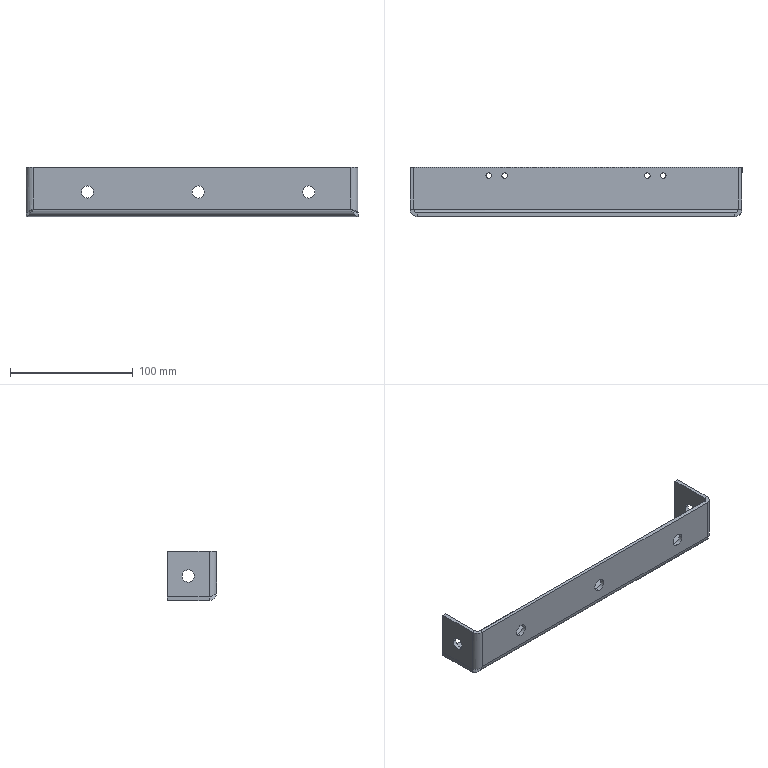Part | SolidWorks | features ICE 2, CornerFeat 1, EdgeFlange 1, FlatPattern 1, SMBaseFlange 1, SheetMetal 1 | 1 solid | 48 faces | box 270 x 40 x 40 mm | volume 67116 mm3 | cylinder 24 | plane 20 | spline 4 | commonest cylinder face diameters 10 x10 4.5 x8 6 x3 12 x3